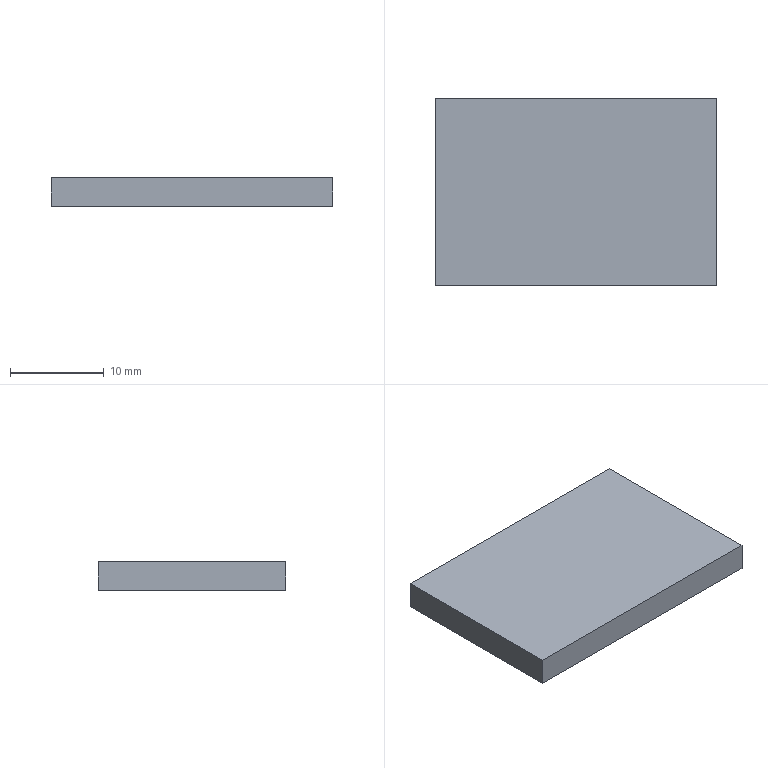Part | STEP file | 5091405 | 1 solid | 6 faces | box 30 x 20 x 3 mm | volume 1800 mm3 | plane 6
STEP:
#1=CARTESIAN_POINT('',(0.,0.,0.));
#2=DIRECTION('',(0.,0.,1.));
#3=DIRECTION('',(1.,0.,0.));
#4=AXIS2_PLACEMENT_3D('',#1,#2,#3);
#5=CARTESIAN_POINT('',(15.,-10.,0.));
#6=VERTEX_POINT('',#5);
#7=CARTESIAN_POINT('',(15.,10.,0.));
#8=VERTEX_POINT('',#7);
#9=CARTESIAN_POINT('',(15.,10.,0.));
#10=DIRECTION('',(0.,1.,0.));
#11=VECTOR('',#10,1.);
#12=LINE('',#9,#11);
#13=CARTESIAN_POINT('',(15.,10.,3.));
#14=DIRECTION('',(-1.,0.,0.));
#15=DIRECTION('',(0.,-1.,0.));
#16=AXIS2_PLACEMENT_3D('',#13,#14,#15);
#17=PLANE('',#16);
#18=CARTESIAN_POINT('',(0.,-3.));
#19=DIRECTION('',(-1.,0.));
#20=VECTOR('',#19,1.);
#21=LINE('',#18,#20);
#22=(GEOMETRIC_REPRESENTATION_CONTEXT(2)PARAMETRIC_REPRESENTATION_CONTEXT()REPRESENTATION_CONTEXT('',''));
#23=DEFINITIONAL_REPRESENTATION('',(#21),#22);
#24=PCURVE('',#17,#23);
#25=CARTESIAN_POINT('',(15.,-10.,0.));
#26=DIRECTION('',(0.,0.,1.));
#27=DIRECTION('',(1.,0.,0.));
#28=AXIS2_PLACEMENT_3D('',#25,#26,#27);
#29=PLANE('',#28);
#30=CARTESIAN_POINT('',(0.,20.));
#31=DIRECTION('',(0.,1.));
#32=VECTOR('',#31,1.);
#33=LINE('',#30,#32);
#34=(GEOMETRIC_REPRESENTATION_CONTEXT(2)PARAMETRIC_REPRESENTATION_CONTEXT()REPRESENTATION_CONTEXT('',''));
#35=DEFINITIONAL_REPRESENTATION('',(#33),#34);
#36=PCURVE('',#29,#35);
#37=SURFACE_CURVE('',#12,(#24,#36),.PCURVE_S1.);
#38=EDGE_CURVE('',#6,#8,#37,.T.);
#39=ORIENTED_EDGE('',*,*,#38,.T.);
#40=CARTESIAN_POINT('',(15.,10.,3.));
#41=VERTEX_POINT('',#40);
#42=CARTESIAN_POINT('',(15.,10.,3.));
#43=DIRECTION('',(0.,0.,-1.));
#44=VECTOR('',#43,1.);
#45=LINE('',#42,#44);
#46=CARTESIAN_POINT('',(0.,0.));
#47=DIRECTION('',(0.,-1.));
#48=VECTOR('',#47,1.);
#49=LINE('',#46,#48);
#50=(GEOMETRIC_REPRESENTATION_CONTEXT(2)PARAMETRIC_REPRESENTATION_CONTEXT()REPRESENTATION_CONTEXT('',''));
#51=DEFINITIONAL_REPRESENTATION('',(#49),#50);
#52=PCURVE('',#17,#51);
#53=CARTESIAN_POINT('',(-15.,10.,3.));
#54=DIRECTION('',(0.,-1.,0.));
#55=DIRECTION('',(0.,0.,-1.));
#56=AXIS2_PLACEMENT_3D('',#53,#54,#55);
#57=PLANE('',#56);
#58=CARTESIAN_POINT('',(0.,30.));
#59=DIRECTION('',(1.,0.));
#60=VECTOR('',#59,1.);
#61=LINE('',#58,#60);
#62=(GEOMETRIC_REPRESENTATION_CONTEXT(2)PARAMETRIC_REPRESENTATION_CONTEXT()REPRESENTATION_CONTEXT('',''));
#63=DEFINITIONAL_REPRESENTATION('',(#61),#62);
#64=PCURVE('',#57,#63);
#65=SURFACE_CURVE('',#45,(#52,#64),.PCURVE_S1.);
#66=EDGE_CURVE('',#41,#8,#65,.T.);
#67=ORIENTED_EDGE('',*,*,#66,.F.);
#68=CARTESIAN_POINT('',(15.,-10.,3.));
#69=VERTEX_POINT('',#68);
#70=CARTESIAN_POINT('',(15.,10.,3.));
#71=DIRECTION('',(0.,1.,0.));
#72=VECTOR('',#71,1.);
#73=LINE('',#70,#72);
#74=CARTESIAN_POINT('',(0.,0.));
#75=DIRECTION('',(-1.,0.));
#76=VECTOR('',#75,1.);
#77=LINE('',#74,#76);
#78=(GEOMETRIC_REPRESENTATION_CONTEXT(2)PARAMETRIC_REPRESENTATION_CONTEXT()REPRESENTATION_CONTEXT('',''));
#79=DEFINITIONAL_REPRESENTATION('',(#77),#78);
#80=PCURVE('',#17,#79);
#81=CARTESIAN_POINT('',(15.,-10.,3.));
#82=DIRECTION('',(0.,0.,1.));
#83=DIRECTION('',(1.,0.,0.));
#84=AXIS2_PLACEMENT_3D('',#81,#82,#83);
#85=PLANE('',#84);
#86=CARTESIAN_POINT('',(0.,20.));
#87=DIRECTION('',(0.,1.));
#88=VECTOR('',#87,1.);
#89=LINE('',#86,#88);
#90=(GEOMETRIC_REPRESENTATION_CONTEXT(2)PARAMETRIC_REPRESENTATION_CONTEXT()REPRESENTATION_CONTEXT('',''));
#91=DEFINITIONAL_REPRESENTATION('',(#89),#90);
#92=PCURVE('',#85,#91);
#93=SURFACE_CURVE('',#73,(#80,#92),.PCURVE_S1.);
#94=EDGE_CURVE('',#69,#41,#93,.T.);
#95=ORIENTED_EDGE('',*,*,#94,.F.);
#96=CARTESIAN_POINT('',(15.,-10.,3.));
#97=DIRECTION('',(0.,0.,-1.));
#98=VECTOR('',#97,1.);
#99=LINE('',#96,#98);
#100=CARTESIAN_POINT('',(20.,0.));
#101=DIRECTION('',(0.,-1.));
#102=VECTOR('',#101,1.);
#103=LINE('',#100,#102);
#104=(GEOMETRIC_REPRESENTATION_CONTEXT(2)PARAMETRIC_REPRESENTATION_CONTEXT()REPRESENTATION_CONTEXT('',''));
#105=DEFINITIONAL_REPRESENTATION('',(#103),#104);
#106=PCURVE('',#17,#105);
#107=CARTESIAN_POINT('',(-15.,-10.,3.));
#108=DIRECTION('',(0.,1.,0.));
#109=DIRECTION('',(0.,0.,1.));
#110=AXIS2_PLACEMENT_3D('',#107,#108,#109);
#111=PLANE('',#110);
#112=CARTESIAN_POINT('',(0.,30.));
#113=DIRECTION('',(-1.,0.));
#114=VECTOR('',#113,1.);
#115=LINE('',#112,#114);
#116=(GEOMETRIC_REPRESENTATION_CONTEXT(2)PARAMETRIC_REPRESENTATION_CONTEXT()REPRESENTATION_CONTEXT('',''));
#117=DEFINITIONAL_REPRESENTATION('',(#115),#116);
#118=PCURVE('',#111,#117);
#119=SURFACE_CURVE('',#99,(#106,#118),.PCURVE_S1.);
#120=EDGE_CURVE('',#69,#6,#119,.T.);
#121=ORIENTED_EDGE('',*,*,#120,.T.);
#122=EDGE_LOOP('',(#39,#67,#95,#121));
#123=FACE_BOUND('',#122,.T.);
#124=ADVANCED_FACE('',(#123),#17,.F.);
#125=CARTESIAN_POINT('',(-15.,10.,0.));
#126=VERTEX_POINT('',#125);
#127=CARTESIAN_POINT('',(-15.,10.,0.));
#128=DIRECTION('',(-1.,0.,0.));
#129=VECTOR('',#128,1.);
#130=LINE('',#127,#129);
#131=CARTESIAN_POINT('',(3.,0.));
#132=DIRECTION('',(0.,-1.));
#133=VECTOR('',#132,1.);
#134=LINE('',#131,#133);
#135=(GEOMETRIC_REPRESENTATION_CONTEXT(2)PARAMETRIC_REPRESENTATION_CONTEXT()REPRESENTATION_CONTEXT('',''));
#136=DEFINITIONAL_REPRESENTATION('',(#134),#135);
#137=PCURVE('',#57,#136);
#138=CARTESIAN_POINT('',(-30.,20.));
#139=DIRECTION('',(-1.,0.));
#140=VECTOR('',#139,1.);
#141=LINE('',#138,#140);
#142=(GEOMETRIC_REPRESENTATION_CONTEXT(2)PARAMETRIC_REPRESENTATION_CONTEXT()REPRESENTATION_CONTEXT('',''));
#143=DEFINITIONAL_REPRESENTATION('',(#141),#142);
#144=PCURVE('',#29,#143);
#145=SURFACE_CURVE('',#130,(#137,#144),.PCURVE_S1.);
#146=EDGE_CURVE('',#8,#126,#145,.T.);
#147=ORIENTED_EDGE('',*,*,#146,.T.);
#148=CARTESIAN_POINT('',(-15.,10.,3.));
#149=VERTEX_POINT('',#148);
#150=CARTESIAN_POINT('',(-15.,10.,3.));
#151=DIRECTION('',(0.,0.,-1.));
#152=VECTOR('',#151,1.);
#153=LINE('',#150,#152);
#154=CARTESIAN_POINT('',(0.,0.));
#155=DIRECTION('',(1.,0.));
#156=VECTOR('',#155,1.);
#157=LINE('',#154,#156);
#158=(GEOMETRIC_REPRESENTATION_CONTEXT(2)PARAMETRIC_REPRESENTATION_CONTEXT()REPRESENTATION_CONTEXT('',''));
#159=DEFINITIONAL_REPRESENTATION('',(#157),#158);
#160=PCURVE('',#57,#159);
#161=CARTESIAN_POINT('',(-15.,10.,3.));
#162=DIRECTION('',(1.,0.,0.));
#163=DIRECTION('',(0.,1.,0.));
#164=AXIS2_PLACEMENT_3D('',#161,#162,#163);
#165=PLANE('',#164);
#166=CARTESIAN_POINT('',(0.,0.));
#167=DIRECTION('',(0.,-1.));
#168=VECTOR('',#167,1.);
#169=LINE('',#166,#168);
#170=(GEOMETRIC_REPRESENTATION_CONTEXT(2)PARAMETRIC_REPRESENTATION_CONTEXT()REPRESENTATION_CONTEXT('',''));
#171=DEFINITIONAL_REPRESENTATION('',(#169),#170);
#172=PCURVE('',#165,#171);
#173=SURFACE_CURVE('',#153,(#160,#172),.PCURVE_S1.);
#174=EDGE_CURVE('',#149,#126,#173,.T.);
#175=ORIENTED_EDGE('',*,*,#174,.F.);
#176=CARTESIAN_POINT('',(-15.,10.,3.));
#177=DIRECTION('',(-1.,0.,0.));
#178=VECTOR('',#177,1.);
#179=LINE('',#176,#178);
#180=CARTESIAN_POINT('',(0.,0.));
#181=DIRECTION('',(0.,-1.));
#182=VECTOR('',#181,1.);
#183=LINE('',#180,#182);
#184=(GEOMETRIC_REPRESENTATION_CONTEXT(2)PARAMETRIC_REPRESENTATION_CONTEXT()REPRESENTATION_CONTEXT('',''));
#185=DEFINITIONAL_REPRESENTATION('',(#183),#184);
#186=PCURVE('',#57,#185);
#187=CARTESIAN_POINT('',(-30.,20.));
#188=DIRECTION('',(-1.,0.));
#189=VECTOR('',#188,1.);
#190=LINE('',#187,#189);
#191=(GEOMETRIC_REPRESENTATION_CONTEXT(2)PARAMETRIC_REPRESENTATION_CONTEXT()REPRESENTATION_CONTEXT('',''));
#192=DEFINITIONAL_REPRESENTATION('',(#190),#191);
#193=PCURVE('',#85,#192);
#194=SURFACE_CURVE('',#179,(#186,#193),.PCURVE_S1.);
#195=EDGE_CURVE('',#41,#149,#194,.T.);
#196=ORIENTED_EDGE('',*,*,#195,.F.);
#197=ORIENTED_EDGE('',*,*,#66,.T.);
#198=EDGE_LOOP('',(#147,#175,#196,#197));
#199=FACE_BOUND('',#198,.T.);
#200=ADVANCED_FACE('',(#199),#57,.F.);
#201=CARTESIAN_POINT('',(-15.,-10.,0.));
#202=VERTEX_POINT('',#201);
#203=CARTESIAN_POINT('',(-15.,10.,0.));
#204=DIRECTION('',(0.,-1.,0.));
#205=VECTOR('',#204,1.);
#206=LINE('',#203,#205);
#207=CARTESIAN_POINT('',(0.,-3.));
#208=DIRECTION('',(-1.,0.));
#209=VECTOR('',#208,1.);
#210=LINE('',#207,#209);
#211=(GEOMETRIC_REPRESENTATION_CONTEXT(2)PARAMETRIC_REPRESENTATION_CONTEXT()REPRESENTATION_CONTEXT('',''));
#212=DEFINITIONAL_REPRESENTATION('',(#210),#211);
#213=PCURVE('',#165,#212);
#214=CARTESIAN_POINT('',(-30.,20.));
#215=DIRECTION('',(0.,-1.));
#216=VECTOR('',#215,1.);
#217=LINE('',#214,#216);
#218=(GEOMETRIC_REPRESENTATION_CONTEXT(2)PARAMETRIC_REPRESENTATION_CONTEXT()REPRESENTATION_CONTEXT('',''));
#219=DEFINITIONAL_REPRESENTATION('',(#217),#218);
#220=PCURVE('',#29,#219);
#221=SURFACE_CURVE('',#206,(#213,#220),.PCURVE_S1.);
#222=EDGE_CURVE('',#126,#202,#221,.T.);
#223=ORIENTED_EDGE('',*,*,#222,.T.);
#224=CARTESIAN_POINT('',(-15.,-10.,3.));
#225=VERTEX_POINT('',#224);
#226=CARTESIAN_POINT('',(-15.,-10.,3.));
#227=DIRECTION('',(0.,0.,-1.));
#228=VECTOR('',#227,1.);
#229=LINE('',#226,#228);
#230=CARTESIAN_POINT('',(-20.,0.));
#231=DIRECTION('',(0.,-1.));
#232=VECTOR('',#231,1.);
#233=LINE('',#230,#232);
#234=(GEOMETRIC_REPRESENTATION_CONTEXT(2)PARAMETRIC_REPRESENTATION_CONTEXT()REPRESENTATION_CONTEXT('',''));
#235=DEFINITIONAL_REPRESENTATION('',(#233),#234);
#236=PCURVE('',#165,#235);
#237=CARTESIAN_POINT('',(0.,0.));
#238=DIRECTION('',(-1.,0.));
#239=VECTOR('',#238,1.);
#240=LINE('',#237,#239);
#241=(GEOMETRIC_REPRESENTATION_CONTEXT(2)PARAMETRIC_REPRESENTATION_CONTEXT()REPRESENTATION_CONTEXT('',''));
#242=DEFINITIONAL_REPRESENTATION('',(#240),#241);
#243=PCURVE('',#111,#242);
#244=SURFACE_CURVE('',#229,(#236,#243),.PCURVE_S1.);
#245=EDGE_CURVE('',#225,#202,#244,.T.);
#246=ORIENTED_EDGE('',*,*,#245,.F.);
#247=CARTESIAN_POINT('',(-15.,10.,3.));
#248=DIRECTION('',(0.,-1.,0.));
#249=VECTOR('',#248,1.);
#250=LINE('',#247,#249);
#251=CARTESIAN_POINT('',(0.,0.));
#252=DIRECTION('',(-1.,0.));
#253=VECTOR('',#252,1.);
#254=LINE('',#251,#253);
#255=(GEOMETRIC_REPRESENTATION_CONTEXT(2)PARAMETRIC_REPRESENTATION_CONTEXT()REPRESENTATION_CONTEXT('',''));
#256=DEFINITIONAL_REPRESENTATION('',(#254),#255);
#257=PCURVE('',#165,#256);
#258=CARTESIAN_POINT('',(-30.,20.));
#259=DIRECTION('',(0.,-1.));
#260=VECTOR('',#259,1.);
#261=LINE('',#258,#260);
#262=(GEOMETRIC_REPRESENTATION_CONTEXT(2)PARAMETRIC_REPRESENTATION_CONTEXT()REPRESENTATION_CONTEXT('',''));
#263=DEFINITIONAL_REPRESENTATION('',(#261),#262);
#264=PCURVE('',#85,#263);
#265=SURFACE_CURVE('',#250,(#257,#264),.PCURVE_S1.);
#266=EDGE_CURVE('',#149,#225,#265,.T.);
#267=ORIENTED_EDGE('',*,*,#266,.F.);
#268=ORIENTED_EDGE('',*,*,#174,.T.);
#269=EDGE_LOOP('',(#223,#246,#267,#268));
#270=FACE_BOUND('',#269,.T.);
#271=ADVANCED_FACE('',(#270),#165,.F.);
#272=CARTESIAN_POINT('',(-15.,-10.,0.));
#273=DIRECTION('',(1.,0.,0.));
#274=VECTOR('',#273,1.);
#275=LINE('',#272,#274);
#276=CARTESIAN_POINT('',(-3.,0.));
#277=DIRECTION('',(0.,1.));
#278=VECTOR('',#277,1.);
#279=LINE('',#276,#278);
#280=(GEOMETRIC_REPRESENTATION_CONTEXT(2)PARAMETRIC_REPRESENTATION_CONTEXT()REPRESENTATION_CONTEXT('',''));
#281=DEFINITIONAL_REPRESENTATION('',(#279),#280);
#282=PCURVE('',#111,#281);
#283=CARTESIAN_POINT('',(-30.,0.));
#284=DIRECTION('',(1.,0.));
#285=VECTOR('',#284,1.);
#286=LINE('',#283,#285);
#287=(GEOMETRIC_REPRESENTATION_CONTEXT(2)PARAMETRIC_REPRESENTATION_CONTEXT()REPRESENTATION_CONTEXT('',''));
#288=DEFINITIONAL_REPRESENTATION('',(#286),#287);
#289=PCURVE('',#29,#288);
#290=SURFACE_CURVE('',#275,(#282,#289),.PCURVE_S1.);
#291=EDGE_CURVE('',#202,#6,#290,.T.);
#292=ORIENTED_EDGE('',*,*,#291,.T.);
#293=ORIENTED_EDGE('',*,*,#120,.F.);
#294=CARTESIAN_POINT('',(-15.,-10.,3.));
#295=DIRECTION('',(1.,0.,0.));
#296=VECTOR('',#295,1.);
#297=LINE('',#294,#296);
#298=CARTESIAN_POINT('',(0.,0.));
#299=DIRECTION('',(0.,1.));
#300=VECTOR('',#299,1.);
#301=LINE('',#298,#300);
#302=(GEOMETRIC_REPRESENTATION_CONTEXT(2)PARAMETRIC_REPRESENTATION_CONTEXT()REPRESENTATION_CONTEXT('',''));
#303=DEFINITIONAL_REPRESENTATION('',(#301),#302);
#304=PCURVE('',#111,#303);
#305=CARTESIAN_POINT('',(-30.,0.));
#306=DIRECTION('',(1.,0.));
#307=VECTOR('',#306,1.);
#308=LINE('',#305,#307);
#309=(GEOMETRIC_REPRESENTATION_CONTEXT(2)PARAMETRIC_REPRESENTATION_CONTEXT()REPRESENTATION_CONTEXT('',''));
#310=DEFINITIONAL_REPRESENTATION('',(#308),#309);
#311=PCURVE('',#85,#310);
#312=SURFACE_CURVE('',#297,(#304,#311),.PCURVE_S1.);
#313=EDGE_CURVE('',#225,#69,#312,.T.);
#314=ORIENTED_EDGE('',*,*,#313,.F.);
#315=ORIENTED_EDGE('',*,*,#245,.T.);
#316=EDGE_LOOP('',(#292,#293,#314,#315));
#317=FACE_BOUND('',#316,.T.);
#318=ADVANCED_FACE('',(#317),#111,.F.);
#319=ORIENTED_EDGE('',*,*,#94,.T.);
#320=ORIENTED_EDGE('',*,*,#195,.T.);
#321=ORIENTED_EDGE('',*,*,#266,.T.);
#322=ORIENTED_EDGE('',*,*,#313,.T.);
#323=EDGE_LOOP('',(#319,#320,#321,#322));
#324=FACE_BOUND('',#323,.T.);
#325=ADVANCED_FACE('',(#324),#85,.T.);
#326=ORIENTED_EDGE('',*,*,#38,.F.);
#327=ORIENTED_EDGE('',*,*,#291,.F.);
#328=ORIENTED_EDGE('',*,*,#222,.F.);
#329=ORIENTED_EDGE('',*,*,#146,.F.);
#330=EDGE_LOOP('',(#326,#327,#328,#329));
#331=FACE_BOUND('',#330,.T.);
#332=ADVANCED_FACE('',(#331),#29,.F.);
#333=CLOSED_SHELL('',(#124,#200,#271,#318,#325,#332));
#334=MANIFOLD_SOLID_BREP('',#333);
#335=(LENGTH_UNIT()NAMED_UNIT(*)SI_UNIT(.MILLI.,.METRE.));
#336=UNCERTAINTY_MEASURE_WITH_UNIT(LENGTH_MEASURE(0.0000001),#335,'','');
#337=(NAMED_UNIT(*)PLANE_ANGLE_UNIT()SI_UNIT($,.RADIAN.));
#338=(NAMED_UNIT(*)SI_UNIT($,.STERADIAN.)SOLID_ANGLE_UNIT());
#339=(GEOMETRIC_REPRESENTATION_CONTEXT(3)GLOBAL_UNCERTAINTY_ASSIGNED_CONTEXT((#336))GLOBAL_UNIT_ASSIGNED_CONTEXT((#335,#337,#338))REPRESENTATION_CONTEXT('',''));
#340=ADVANCED_BREP_SHAPE_REPRESENTATION('',(#4,#334),#339);